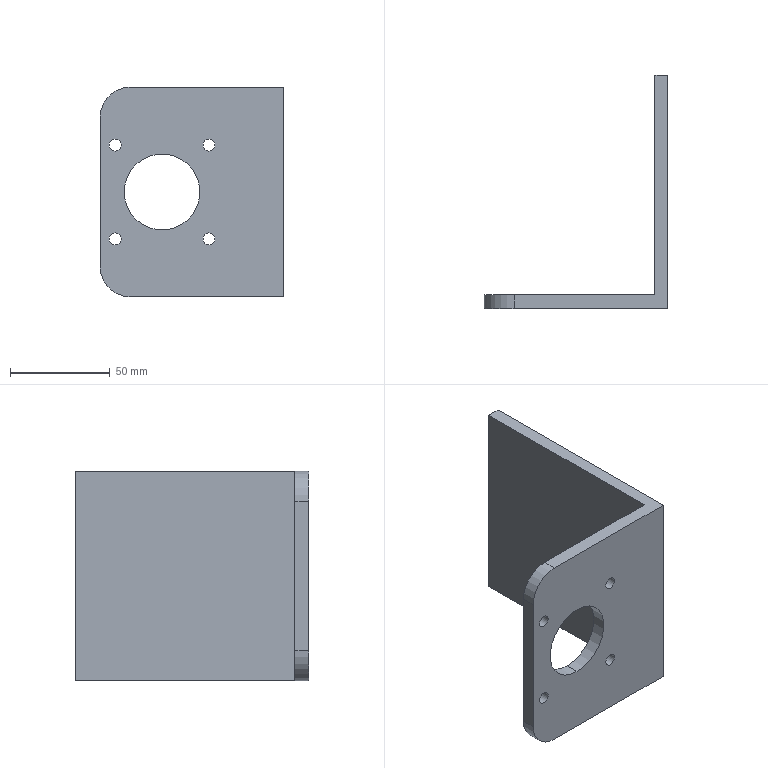Part | NX | 1 solid | 16 faces | box 92 x 117 x 105 mm | volume 132849 mm3 | plane 8 | cylinder 8 | commonest cylinder face diameters 6 x4 30 x2 38 x2
STEP:
#1=CARTESIAN_POINT('',(5305.429,392.144,-335.119));
#2=VERTEX_POINT('',#1);
#3=CARTESIAN_POINT('',(5305.429,392.144,-332.119));
#4=DIRECTION('',(0.,1.,0.));
#5=DIRECTION('',(0.,0.,-1.));
#6=AXIS2_PLACEMENT_3D('',#3,#4,#5);
#7=CIRCLE('',#6,3.);
#8=EDGE_CURVE('',#2,#2,#7,.T.);
#9=ORIENTED_EDGE('',*,*,#8,.F.);
#10=EDGE_LOOP('',(#9));
#11=FACE_BOUND('',#10,.T.);
#12=CARTESIAN_POINT('',(5258.429,392.144,-288.119));
#13=VERTEX_POINT('',#12);
#14=CARTESIAN_POINT('',(5258.429,392.144,-285.119));
#15=DIRECTION('',(0.,1.,0.));
#16=DIRECTION('',(0.,0.,-1.));
#17=AXIS2_PLACEMENT_3D('',#14,#15,#16);
#18=CIRCLE('',#17,3.);
#19=EDGE_CURVE('',#13,#13,#18,.T.);
#20=ORIENTED_EDGE('',*,*,#19,.F.);
#21=EDGE_LOOP('',(#20));
#22=FACE_BOUND('',#21,.T.);
#23=CARTESIAN_POINT('',(5258.429,392.144,-335.119));
#24=VERTEX_POINT('',#23);
#25=CARTESIAN_POINT('',(5258.429,392.144,-332.119));
#26=DIRECTION('',(0.,1.,0.));
#27=DIRECTION('',(0.,0.,-1.));
#28=AXIS2_PLACEMENT_3D('',#25,#26,#27);
#29=CIRCLE('',#28,3.);
#30=EDGE_CURVE('',#24,#24,#29,.T.);
#31=ORIENTED_EDGE('',*,*,#30,.F.);
#32=EDGE_LOOP('',(#31));
#33=FACE_BOUND('',#32,.T.);
#34=CARTESIAN_POINT('',(5305.429,392.144,-288.119));
#35=VERTEX_POINT('',#34);
#36=CARTESIAN_POINT('',(5305.429,392.144,-285.119));
#37=DIRECTION('',(0.,1.,0.));
#38=DIRECTION('',(0.,0.,-1.));
#39=AXIS2_PLACEMENT_3D('',#36,#37,#38);
#40=CIRCLE('',#39,3.);
#41=EDGE_CURVE('',#35,#35,#40,.T.);
#42=ORIENTED_EDGE('',*,*,#41,.F.);
#43=EDGE_LOOP('',(#42));
#44=FACE_BOUND('',#43,.T.);
#45=CARTESIAN_POINT('',(5336.467,392.144,-361.119));
#46=VERTEX_POINT('',#45);
#47=CARTESIAN_POINT('',(5265.929,392.144,-361.119));
#48=VERTEX_POINT('',#47);
#49=CARTESIAN_POINT('',(5250.929,392.144,-361.119));
#50=DIRECTION('',(-1.,0.,0.));
#51=VECTOR('',#50,1.);
#52=LINE('',#49,#51);
#53=EDGE_CURVE('',#46,#48,#52,.T.);
#54=ORIENTED_EDGE('',*,*,#53,.T.);
#55=CARTESIAN_POINT('',(5250.929,392.144,-346.119));
#56=VERTEX_POINT('',#55);
#57=CARTESIAN_POINT('',(5265.929,392.144,-346.119));
#58=DIRECTION('',(0.,1.,0.));
#59=DIRECTION('',(0.,0.,-1.));
#60=AXIS2_PLACEMENT_3D('',#57,#58,#59);
#61=CIRCLE('',#60,15.);
#62=EDGE_CURVE('',#48,#56,#61,.T.);
#63=ORIENTED_EDGE('',*,*,#62,.T.);
#64=CARTESIAN_POINT('',(5250.929,392.144,-271.119));
#65=VERTEX_POINT('',#64);
#66=CARTESIAN_POINT('',(5250.929,392.144,-1295.619));
#67=DIRECTION('',(0.,0.,1.));
#68=VECTOR('',#67,1.);
#69=LINE('',#66,#68);
#70=EDGE_CURVE('',#56,#65,#69,.T.);
#71=ORIENTED_EDGE('',*,*,#70,.T.);
#72=CARTESIAN_POINT('',(5265.929,392.144,-256.119));
#73=VERTEX_POINT('',#72);
#74=CARTESIAN_POINT('',(5265.929,392.144,-271.119));
#75=DIRECTION('',(0.,1.,0.));
#76=DIRECTION('',(0.,0.,-1.));
#77=AXIS2_PLACEMENT_3D('',#74,#75,#76);
#78=CIRCLE('',#77,15.);
#79=EDGE_CURVE('',#65,#73,#78,.T.);
#80=ORIENTED_EDGE('',*,*,#79,.T.);
#81=CARTESIAN_POINT('',(5336.467,392.144,-256.119));
#82=VERTEX_POINT('',#81);
#83=CARTESIAN_POINT('',(5250.929,392.144,-256.119));
#84=DIRECTION('',(1.,0.,0.));
#85=VECTOR('',#84,1.);
#86=LINE('',#83,#85);
#87=EDGE_CURVE('',#73,#82,#86,.T.);
#88=ORIENTED_EDGE('',*,*,#87,.T.);
#89=CARTESIAN_POINT('',(5336.467,392.144,-1295.619));
#90=DIRECTION('',(0.,0.,1.));
#91=VECTOR('',#90,1.);
#92=LINE('',#89,#91);
#93=EDGE_CURVE('',#46,#82,#92,.T.);
#94=ORIENTED_EDGE('',*,*,#93,.F.);
#95=EDGE_LOOP('',(#54,#63,#71,#80,#88,#94));
#96=FACE_BOUND('',#95,.T.);
#97=CARTESIAN_POINT('',(5281.929,392.144,-327.619));
#98=VERTEX_POINT('',#97);
#99=CARTESIAN_POINT('',(5281.929,392.144,-289.619));
#100=VERTEX_POINT('',#99);
#101=CARTESIAN_POINT('',(5281.929,392.144,-308.619));
#102=DIRECTION('',(0.,-1.,0.));
#103=DIRECTION('',(-1.,0.,0.));
#104=AXIS2_PLACEMENT_3D('',#101,#102,#103);
#105=CIRCLE('',#104,19.);
#106=EDGE_CURVE('',#98,#100,#105,.T.);
#107=ORIENTED_EDGE('',*,*,#106,.T.);
#108=CARTESIAN_POINT('',(5281.929,392.144,-308.619));
#109=DIRECTION('',(0.,-1.,0.));
#110=DIRECTION('',(-1.,0.,0.));
#111=AXIS2_PLACEMENT_3D('',#108,#109,#110);
#112=CIRCLE('',#111,19.);
#113=EDGE_CURVE('',#100,#98,#112,.T.);
#114=ORIENTED_EDGE('',*,*,#113,.T.);
#115=EDGE_LOOP('',(#107,#114));
#116=FACE_BOUND('',#115,.T.);
#117=CARTESIAN_POINT('',(5250.929,392.144,-1295.619));
#118=DIRECTION('',(0.,-1.,0.));
#119=DIRECTION('',(0.,0.,-1.));
#120=AXIS2_PLACEMENT_3D('',#117,#118,#119);
#121=PLANE('',#120);
#122=ADVANCED_FACE('',(#11,#22,#33,#44,#96,#116),#121,.F.);
#123=CARTESIAN_POINT('',(5265.929,385.144,-361.119));
#124=VERTEX_POINT('',#123);
#125=CARTESIAN_POINT('',(5342.929,385.144,-361.119));
#126=VERTEX_POINT('',#125);
#127=CARTESIAN_POINT('',(5342.929,385.144,-361.119));
#128=DIRECTION('',(1.,0.,0.));
#129=VECTOR('',#128,1.);
#130=LINE('',#127,#129);
#131=EDGE_CURVE('',#124,#126,#130,.T.);
#132=ORIENTED_EDGE('',*,*,#131,.F.);
#133=CARTESIAN_POINT('',(5265.929,392.144,-361.119));
#134=DIRECTION('',(0.,1.,0.));
#135=VECTOR('',#134,1.);
#136=LINE('',#133,#135);
#137=EDGE_CURVE('',#124,#48,#136,.T.);
#138=ORIENTED_EDGE('',*,*,#137,.T.);
#139=ORIENTED_EDGE('',*,*,#53,.F.);
#140=CARTESIAN_POINT('',(5336.467,502.144,-361.119));
#141=VERTEX_POINT('',#140);
#142=CARTESIAN_POINT('',(5336.467,392.144,-361.119));
#143=DIRECTION('',(0.,-1.,0.));
#144=VECTOR('',#143,1.);
#145=LINE('',#142,#144);
#146=EDGE_CURVE('',#141,#46,#145,.T.);
#147=ORIENTED_EDGE('',*,*,#146,.F.);
#148=CARTESIAN_POINT('',(5342.929,502.144,-361.119));
#149=VERTEX_POINT('',#148);
#150=CARTESIAN_POINT('',(5336.467,502.144,-361.119));
#151=DIRECTION('',(-1.,0.,0.));
#152=VECTOR('',#151,1.);
#153=LINE('',#150,#152);
#154=EDGE_CURVE('',#149,#141,#153,.T.);
#155=ORIENTED_EDGE('',*,*,#154,.F.);
#156=CARTESIAN_POINT('',(5342.929,502.144,-361.119));
#157=DIRECTION('',(0.,1.,0.));
#158=VECTOR('',#157,1.);
#159=LINE('',#156,#158);
#160=EDGE_CURVE('',#126,#149,#159,.T.);
#161=ORIENTED_EDGE('',*,*,#160,.F.);
#162=EDGE_LOOP('',(#132,#138,#139,#147,#155,#161));
#163=FACE_OUTER_BOUND('',#162,.T.);
#164=CARTESIAN_POINT('',(5352.929,392.144,-361.119));
#165=DIRECTION('',(0.,0.,1.));
#166=DIRECTION('',(0.,-1.,0.));
#167=AXIS2_PLACEMENT_3D('',#164,#165,#166);
#168=PLANE('',#167);
#169=ADVANCED_FACE('',(#163),#168,.F.);
#170=ORIENTED_EDGE('',*,*,#70,.F.);
#171=CARTESIAN_POINT('',(5250.929,385.144,-346.119));
#172=VERTEX_POINT('',#171);
#173=CARTESIAN_POINT('',(5250.929,385.144,-346.119));
#174=DIRECTION('',(0.,-1.,0.));
#175=VECTOR('',#174,1.);
#176=LINE('',#173,#175);
#177=EDGE_CURVE('',#56,#172,#176,.T.);
#178=ORIENTED_EDGE('',*,*,#177,.T.);
#179=CARTESIAN_POINT('',(5250.929,385.144,-271.119));
#180=VERTEX_POINT('',#179);
#181=CARTESIAN_POINT('',(5250.929,385.144,-1295.619));
#182=DIRECTION('',(0.,0.,1.));
#183=VECTOR('',#182,1.);
#184=LINE('',#181,#183);
#185=EDGE_CURVE('',#172,#180,#184,.T.);
#186=ORIENTED_EDGE('',*,*,#185,.T.);
#187=CARTESIAN_POINT('',(5250.929,385.144,-271.119));
#188=DIRECTION('',(0.,1.,0.));
#189=VECTOR('',#188,1.);
#190=LINE('',#187,#189);
#191=EDGE_CURVE('',#180,#65,#190,.T.);
#192=ORIENTED_EDGE('',*,*,#191,.T.);
#193=EDGE_LOOP('',(#170,#178,#186,#192));
#194=FACE_OUTER_BOUND('',#193,.T.);
#195=CARTESIAN_POINT('',(5250.929,385.144,-1295.619));
#196=DIRECTION('',(1.,0.,0.));
#197=DIRECTION('',(0.,0.,-1.));
#198=AXIS2_PLACEMENT_3D('',#195,#196,#197);
#199=PLANE('',#198);
#200=ADVANCED_FACE('',(#194),#199,.F.);
#201=CARTESIAN_POINT('',(5336.467,502.144,-256.119));
#202=VERTEX_POINT('',#201);
#203=CARTESIAN_POINT('',(5336.467,502.144,-1295.619));
#204=DIRECTION('',(0.,0.,1.));
#205=VECTOR('',#204,1.);
#206=LINE('',#203,#205);
#207=EDGE_CURVE('',#141,#202,#206,.T.);
#208=ORIENTED_EDGE('',*,*,#207,.F.);
#209=ORIENTED_EDGE('',*,*,#146,.T.);
#210=ORIENTED_EDGE('',*,*,#93,.T.);
#211=CARTESIAN_POINT('',(5336.467,392.144,-256.119));
#212=DIRECTION('',(0.,1.,0.));
#213=VECTOR('',#212,1.);
#214=LINE('',#211,#213);
#215=EDGE_CURVE('',#82,#202,#214,.T.);
#216=ORIENTED_EDGE('',*,*,#215,.T.);
#217=EDGE_LOOP('',(#208,#209,#210,#216));
#218=FACE_OUTER_BOUND('',#217,.T.);
#219=CARTESIAN_POINT('',(5336.467,392.144,-1295.619));
#220=DIRECTION('',(1.,0.,0.));
#221=DIRECTION('',(0.,0.,-1.));
#222=AXIS2_PLACEMENT_3D('',#219,#220,#221);
#223=PLANE('',#222);
#224=ADVANCED_FACE('',(#218),#223,.F.);
#225=ORIENTED_EDGE('',*,*,#87,.F.);
#226=CARTESIAN_POINT('',(5265.929,385.144,-256.119));
#227=VERTEX_POINT('',#226);
#228=CARTESIAN_POINT('',(5265.929,0.,-256.119));
#229=DIRECTION('',(0.,-1.,0.));
#230=VECTOR('',#229,1.);
#231=LINE('',#228,#230);
#232=EDGE_CURVE('',#73,#227,#231,.T.);
#233=ORIENTED_EDGE('',*,*,#232,.T.);
#234=CARTESIAN_POINT('',(5342.929,385.144,-256.119));
#235=VERTEX_POINT('',#234);
#236=CARTESIAN_POINT('',(5342.929,385.144,-256.119));
#237=DIRECTION('',(-1.,0.,0.));
#238=VECTOR('',#237,1.);
#239=LINE('',#236,#238);
#240=EDGE_CURVE('',#235,#227,#239,.T.);
#241=ORIENTED_EDGE('',*,*,#240,.F.);
#242=CARTESIAN_POINT('',(5342.929,502.144,-256.119));
#243=VERTEX_POINT('',#242);
#244=CARTESIAN_POINT('',(5342.929,502.144,-256.119));
#245=DIRECTION('',(0.,-1.,0.));
#246=VECTOR('',#245,1.);
#247=LINE('',#244,#246);
#248=EDGE_CURVE('',#243,#235,#247,.T.);
#249=ORIENTED_EDGE('',*,*,#248,.F.);
#250=CARTESIAN_POINT('',(5336.467,502.144,-256.119));
#251=DIRECTION('',(1.,0.,0.));
#252=VECTOR('',#251,1.);
#253=LINE('',#250,#252);
#254=EDGE_CURVE('',#202,#243,#253,.T.);
#255=ORIENTED_EDGE('',*,*,#254,.F.);
#256=ORIENTED_EDGE('',*,*,#215,.F.);
#257=EDGE_LOOP('',(#225,#233,#241,#249,#255,#256));
#258=FACE_OUTER_BOUND('',#257,.T.);
#259=CARTESIAN_POINT('',(0.,0.,-256.119));
#260=DIRECTION('',(0.,0.,-1.));
#261=DIRECTION('',(-1.,0.,0.));
#262=AXIS2_PLACEMENT_3D('',#259,#260,#261);
#263=PLANE('',#262);
#264=ADVANCED_FACE('',(#258),#263,.F.);
#265=CARTESIAN_POINT('',(5342.929,502.144,-1295.619));
#266=DIRECTION('',(0.,0.,1.));
#267=VECTOR('',#266,1.);
#268=LINE('',#265,#267);
#269=EDGE_CURVE('',#149,#243,#268,.T.);
#270=ORIENTED_EDGE('',*,*,#269,.F.);
#271=ORIENTED_EDGE('',*,*,#154,.T.);
#272=ORIENTED_EDGE('',*,*,#207,.T.);
#273=ORIENTED_EDGE('',*,*,#254,.T.);
#274=EDGE_LOOP('',(#270,#271,#272,#273));
#275=FACE_OUTER_BOUND('',#274,.T.);
#276=CARTESIAN_POINT('',(5336.467,502.144,-1295.619));
#277=DIRECTION('',(0.,-1.,0.));
#278=DIRECTION('',(0.,0.,-1.));
#279=AXIS2_PLACEMENT_3D('',#276,#277,#278);
#280=PLANE('',#279);
#281=ADVANCED_FACE('',(#275),#280,.F.);
#282=CARTESIAN_POINT('',(5305.429,385.144,-329.119));
#283=VERTEX_POINT('',#282);
#284=CARTESIAN_POINT('',(5305.429,385.144,-332.119));
#285=DIRECTION('',(0.,-1.,0.));
#286=DIRECTION('',(0.,0.,1.));
#287=AXIS2_PLACEMENT_3D('',#284,#285,#286);
#288=CIRCLE('',#287,3.);
#289=EDGE_CURVE('',#283,#283,#288,.T.);
#290=ORIENTED_EDGE('',*,*,#289,.F.);
#291=EDGE_LOOP('',(#290));
#292=FACE_BOUND('',#291,.T.);
#293=CARTESIAN_POINT('',(5258.429,385.144,-282.119));
#294=VERTEX_POINT('',#293);
#295=CARTESIAN_POINT('',(5258.429,385.144,-285.119));
#296=DIRECTION('',(0.,-1.,0.));
#297=DIRECTION('',(0.,0.,1.));
#298=AXIS2_PLACEMENT_3D('',#295,#296,#297);
#299=CIRCLE('',#298,3.);
#300=EDGE_CURVE('',#294,#294,#299,.T.);
#301=ORIENTED_EDGE('',*,*,#300,.F.);
#302=EDGE_LOOP('',(#301));
#303=FACE_BOUND('',#302,.T.);
#304=CARTESIAN_POINT('',(5258.429,385.144,-329.119));
#305=VERTEX_POINT('',#304);
#306=CARTESIAN_POINT('',(5258.429,385.144,-332.119));
#307=DIRECTION('',(0.,-1.,0.));
#308=DIRECTION('',(0.,0.,1.));
#309=AXIS2_PLACEMENT_3D('',#306,#307,#308);
#310=CIRCLE('',#309,3.);
#311=EDGE_CURVE('',#305,#305,#310,.T.);
#312=ORIENTED_EDGE('',*,*,#311,.F.);
#313=EDGE_LOOP('',(#312));
#314=FACE_BOUND('',#313,.T.);
#315=CARTESIAN_POINT('',(5305.429,385.144,-282.119));
#316=VERTEX_POINT('',#315);
#317=CARTESIAN_POINT('',(5305.429,385.144,-285.119));
#318=DIRECTION('',(0.,-1.,0.));
#319=DIRECTION('',(0.,0.,1.));
#320=AXIS2_PLACEMENT_3D('',#317,#318,#319);
#321=CIRCLE('',#320,3.);
#322=EDGE_CURVE('',#316,#316,#321,.T.);
#323=ORIENTED_EDGE('',*,*,#322,.F.);
#324=EDGE_LOOP('',(#323));
#325=FACE_BOUND('',#324,.T.);
#326=CARTESIAN_POINT('',(5281.929,385.144,-289.619));
#327=VERTEX_POINT('',#326);
#328=CARTESIAN_POINT('',(5281.929,385.144,-327.619));
#329=VERTEX_POINT('',#328);
#330=CARTESIAN_POINT('',(5281.929,385.144,-308.619));
#331=DIRECTION('',(0.,1.,0.));
#332=DIRECTION('',(0.,0.,1.));
#333=AXIS2_PLACEMENT_3D('',#330,#331,#332);
#334=CIRCLE('',#333,19.);
#335=EDGE_CURVE('',#327,#329,#334,.T.);
#336=ORIENTED_EDGE('',*,*,#335,.T.);
#337=CARTESIAN_POINT('',(5281.929,385.144,-308.619));
#338=DIRECTION('',(0.,1.,0.));
#339=DIRECTION('',(0.,0.,1.));
#340=AXIS2_PLACEMENT_3D('',#337,#338,#339);
#341=CIRCLE('',#340,19.);
#342=EDGE_CURVE('',#329,#327,#341,.T.);
#343=ORIENTED_EDGE('',*,*,#342,.T.);
#344=EDGE_LOOP('',(#336,#343));
#345=FACE_BOUND('',#344,.T.);
#346=ORIENTED_EDGE('',*,*,#185,.F.);
#347=CARTESIAN_POINT('',(5265.929,385.144,-346.119));
#348=DIRECTION('',(0.,-1.,0.));
#349=DIRECTION('',(0.,0.,1.));
#350=AXIS2_PLACEMENT_3D('',#347,#348,#349);
#351=CIRCLE('',#350,15.);
#352=EDGE_CURVE('',#172,#124,#351,.T.);
#353=ORIENTED_EDGE('',*,*,#352,.T.);
#354=ORIENTED_EDGE('',*,*,#131,.T.);
#355=CARTESIAN_POINT('',(5342.929,385.144,-1295.619));
#356=DIRECTION('',(0.,0.,1.));
#357=VECTOR('',#356,1.);
#358=LINE('',#355,#357);
#359=EDGE_CURVE('',#126,#235,#358,.T.);
#360=ORIENTED_EDGE('',*,*,#359,.T.);
#361=ORIENTED_EDGE('',*,*,#240,.T.);
#362=CARTESIAN_POINT('',(5265.929,385.144,-271.119));
#363=DIRECTION('',(0.,-1.,0.));
#364=DIRECTION('',(0.,0.,1.));
#365=AXIS2_PLACEMENT_3D('',#362,#363,#364);
#366=CIRCLE('',#365,15.);
#367=EDGE_CURVE('',#227,#180,#366,.T.);
#368=ORIENTED_EDGE('',*,*,#367,.T.);
#369=EDGE_LOOP('',(#346,#353,#354,#360,#361,#368));
#370=FACE_BOUND('',#369,.T.);
#371=CARTESIAN_POINT('',(5342.929,385.144,-1295.619));
#372=DIRECTION('',(0.,1.,0.));
#373=DIRECTION('',(0.,0.,1.));
#374=AXIS2_PLACEMENT_3D('',#371,#372,#373);
#375=PLANE('',#374);
#376=ADVANCED_FACE('',(#292,#303,#314,#325,#345,#370),#375,.F.);
#377=ORIENTED_EDGE('',*,*,#359,.F.);
#378=ORIENTED_EDGE('',*,*,#160,.T.);
#379=ORIENTED_EDGE('',*,*,#269,.T.);
#380=ORIENTED_EDGE('',*,*,#248,.T.);
#381=EDGE_LOOP('',(#377,#378,#379,#380));
#382=FACE_OUTER_BOUND('',#381,.T.);
#383=CARTESIAN_POINT('',(5342.929,502.144,-1295.619));
#384=DIRECTION('',(-1.,0.,0.));
#385=DIRECTION('',(0.,0.,1.));
#386=AXIS2_PLACEMENT_3D('',#383,#384,#385);
#387=PLANE('',#386);
#388=ADVANCED_FACE('',(#382),#387,.F.);
#389=ORIENTED_EDGE('',*,*,#113,.F.);
#390=CARTESIAN_POINT('',(5281.929,392.644,-289.619));
#391=DIRECTION('',(0.,1.,0.));
#392=VECTOR('',#391,1.);
#393=LINE('',#390,#392);
#394=EDGE_CURVE('',#327,#100,#393,.T.);
#395=ORIENTED_EDGE('',*,*,#394,.F.);
#396=ORIENTED_EDGE('',*,*,#342,.F.);
#397=CARTESIAN_POINT('',(5281.929,392.644,-327.619));
#398=DIRECTION('',(0.,-1.,0.));
#399=VECTOR('',#398,1.);
#400=LINE('',#397,#399);
#401=EDGE_CURVE('',#98,#329,#400,.T.);
#402=ORIENTED_EDGE('',*,*,#401,.F.);
#403=EDGE_LOOP('',(#389,#395,#396,#402));
#404=FACE_OUTER_BOUND('',#403,.T.);
#405=CARTESIAN_POINT('',(5281.929,392.644,-308.619));
#406=DIRECTION('',(0.,1.,0.));
#407=DIRECTION('',(0.,0.,1.));
#408=AXIS2_PLACEMENT_3D('',#405,#406,#407);
#409=CYLINDRICAL_SURFACE('',#408,19.);
#410=ADVANCED_FACE('',(#404),#409,.F.);
#411=ORIENTED_EDGE('',*,*,#106,.F.);
#412=ORIENTED_EDGE('',*,*,#401,.T.);
#413=ORIENTED_EDGE('',*,*,#335,.F.);
#414=ORIENTED_EDGE('',*,*,#394,.T.);
#415=EDGE_LOOP('',(#411,#412,#413,#414));
#416=FACE_OUTER_BOUND('',#415,.T.);
#417=CARTESIAN_POINT('',(5281.929,392.644,-308.619));
#418=DIRECTION('',(0.,1.,0.));
#419=DIRECTION('',(0.,0.,1.));
#420=AXIS2_PLACEMENT_3D('',#417,#418,#419);
#421=CYLINDRICAL_SURFACE('',#420,19.);
#422=ADVANCED_FACE('',(#416),#421,.F.);
#423=ORIENTED_EDGE('',*,*,#62,.F.);
#424=ORIENTED_EDGE('',*,*,#137,.F.);
#425=ORIENTED_EDGE('',*,*,#352,.F.);
#426=ORIENTED_EDGE('',*,*,#177,.F.);
#427=EDGE_LOOP('',(#423,#424,#425,#426));
#428=FACE_OUTER_BOUND('',#427,.T.);
#429=CARTESIAN_POINT('',(5265.929,385.144,-346.119));
#430=DIRECTION('',(0.,-1.,0.));
#431=DIRECTION('',(0.,0.,-1.));
#432=AXIS2_PLACEMENT_3D('',#429,#430,#431);
#433=CYLINDRICAL_SURFACE('',#432,15.);
#434=ADVANCED_FACE('',(#428),#433,.T.);
#435=ORIENTED_EDGE('',*,*,#367,.F.);
#436=ORIENTED_EDGE('',*,*,#232,.F.);
#437=ORIENTED_EDGE('',*,*,#79,.F.);
#438=ORIENTED_EDGE('',*,*,#191,.F.);
#439=EDGE_LOOP('',(#435,#436,#437,#438));
#440=FACE_OUTER_BOUND('',#439,.T.);
#441=CARTESIAN_POINT('',(5265.929,385.144,-271.119));
#442=DIRECTION('',(0.,1.,0.));
#443=DIRECTION('',(0.,0.,1.));
#444=AXIS2_PLACEMENT_3D('',#441,#442,#443);
#445=CYLINDRICAL_SURFACE('',#444,15.);
#446=ADVANCED_FACE('',(#440),#445,.T.);
#447=ORIENTED_EDGE('',*,*,#322,.T.);
#448=EDGE_LOOP('',(#447));
#449=FACE_BOUND('',#448,.T.);
#450=ORIENTED_EDGE('',*,*,#41,.T.);
#451=EDGE_LOOP('',(#450));
#452=FACE_BOUND('',#451,.T.);
#453=CARTESIAN_POINT('',(5305.429,497.144,-285.119));
#454=DIRECTION('',(0.,-1.,0.));
#455=DIRECTION('',(0.,0.,-1.));
#456=AXIS2_PLACEMENT_3D('',#453,#454,#455);
#457=CYLINDRICAL_SURFACE('',#456,3.);
#458=ADVANCED_FACE('',(#449,#452),#457,.F.);
#459=ORIENTED_EDGE('',*,*,#311,.T.);
#460=EDGE_LOOP('',(#459));
#461=FACE_BOUND('',#460,.T.);
#462=ORIENTED_EDGE('',*,*,#30,.T.);
#463=EDGE_LOOP('',(#462));
#464=FACE_BOUND('',#463,.T.);
#465=CARTESIAN_POINT('',(5258.429,497.144,-332.119));
#466=DIRECTION('',(0.,-1.,0.));
#467=DIRECTION('',(0.,0.,-1.));
#468=AXIS2_PLACEMENT_3D('',#465,#466,#467);
#469=CYLINDRICAL_SURFACE('',#468,3.);
#470=ADVANCED_FACE('',(#461,#464),#469,.F.);
#471=ORIENTED_EDGE('',*,*,#300,.T.);
#472=EDGE_LOOP('',(#471));
#473=FACE_BOUND('',#472,.T.);
#474=ORIENTED_EDGE('',*,*,#19,.T.);
#475=EDGE_LOOP('',(#474));
#476=FACE_BOUND('',#475,.T.);
#477=CARTESIAN_POINT('',(5258.429,497.144,-285.119));
#478=DIRECTION('',(0.,-1.,0.));
#479=DIRECTION('',(0.,0.,-1.));
#480=AXIS2_PLACEMENT_3D('',#477,#478,#479);
#481=CYLINDRICAL_SURFACE('',#480,3.);
#482=ADVANCED_FACE('',(#473,#476),#481,.F.);
#483=ORIENTED_EDGE('',*,*,#289,.T.);
#484=EDGE_LOOP('',(#483));
#485=FACE_BOUND('',#484,.T.);
#486=ORIENTED_EDGE('',*,*,#8,.T.);
#487=EDGE_LOOP('',(#486));
#488=FACE_BOUND('',#487,.T.);
#489=CARTESIAN_POINT('',(5305.429,497.144,-332.119));
#490=DIRECTION('',(0.,-1.,0.));
#491=DIRECTION('',(0.,0.,-1.));
#492=AXIS2_PLACEMENT_3D('',#489,#490,#491);
#493=CYLINDRICAL_SURFACE('',#492,3.);
#494=ADVANCED_FACE('',(#485,#488),#493,.F.);
#495=CLOSED_SHELL('',(#122,#169,#200,#224,#264,#281,#376,#388,#410,#422,#434,#446,#458,#470,#482,#494));
#496=MANIFOLD_SOLID_BREP('',#495);
#497=(LENGTH_UNIT()NAMED_UNIT(*)SI_UNIT(.MILLI.,.METRE.));
#498=UNCERTAINTY_MEASURE_WITH_UNIT(LENGTH_MEASURE(0.00002),#497,'','');
#499=(NAMED_UNIT(*)PLANE_ANGLE_UNIT()SI_UNIT($,.RADIAN.));
#500=PLANE_ANGLE_MEASURE_WITH_UNIT(PLANE_ANGLE_MEASURE(0.01745),#499);
#501=DIMENSIONAL_EXPONENTS(0.,0.,0.,0.,0.,0.,0.);
#502=(CONVERSION_BASED_UNIT('DEGREE',#500)NAMED_UNIT(#501)PLANE_ANGLE_UNIT());
#503=(NAMED_UNIT(*)SI_UNIT($,.STERADIAN.)SOLID_ANGLE_UNIT());
#504=(GEOMETRIC_REPRESENTATION_CONTEXT(3)GLOBAL_UNCERTAINTY_ASSIGNED_CONTEXT((#498))GLOBAL_UNIT_ASSIGNED_CONTEXT((#497,#502,#503))REPRESENTATION_CONTEXT('',''));
#505=ADVANCED_BREP_SHAPE_REPRESENTATION('',(#496),#504);